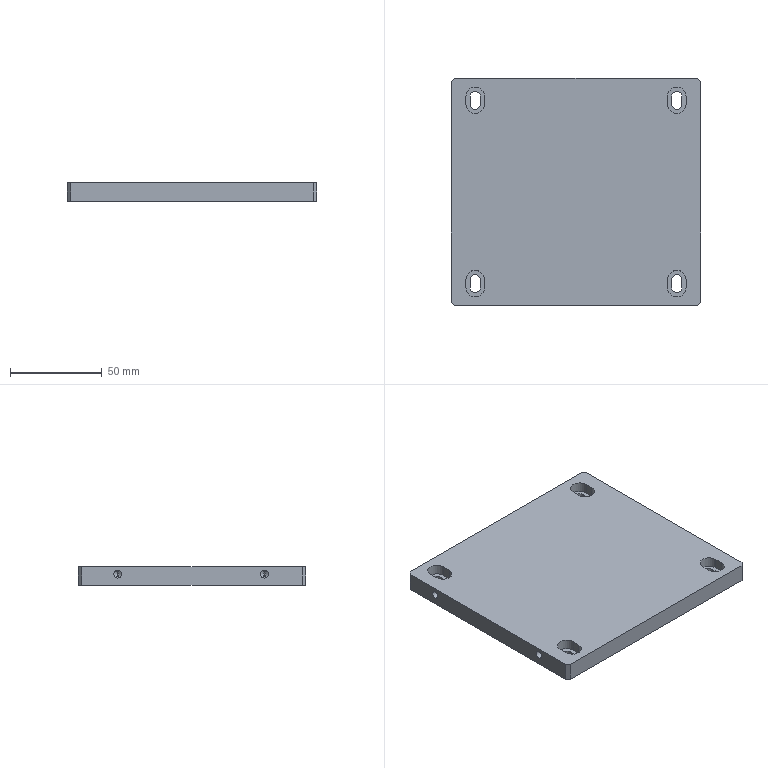Part | STEP file | FBDS-ZUO | 1 solid | 62 faces | box 136 x 124 x 10 mm | volume 164198 mm3 | plane 30 | cylinder 24 | cone 8 | commonest cylinder face diameters 4.2 x8 5.5 x8 10 x8